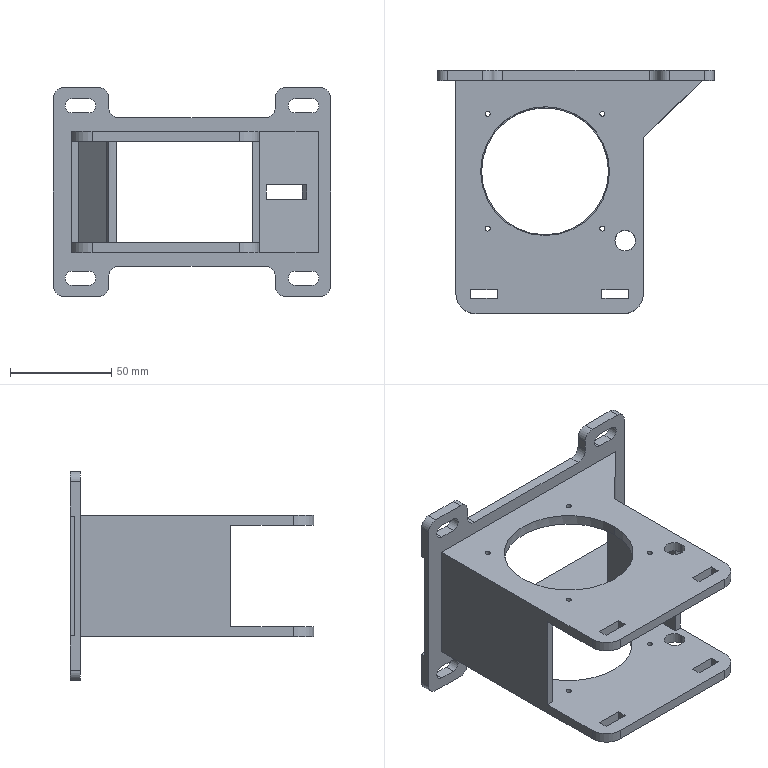Part | NX | features DATUM_CSYS 2, EXTRUDE 2, SKETCH 2, BREP 1, EXTRACT_DATUM_PLANE 1, INTERSECT 1, UNITE 1 | 1 solid | 114 faces | box 136.5 x 120 x 103 mm | volume 129475 mm3 | plane 66 | cylinder 48 | commonest cylinder face diameters 2.5 x16 10 x12 7 x8 10.2 x4 20 x4 62.5 x2